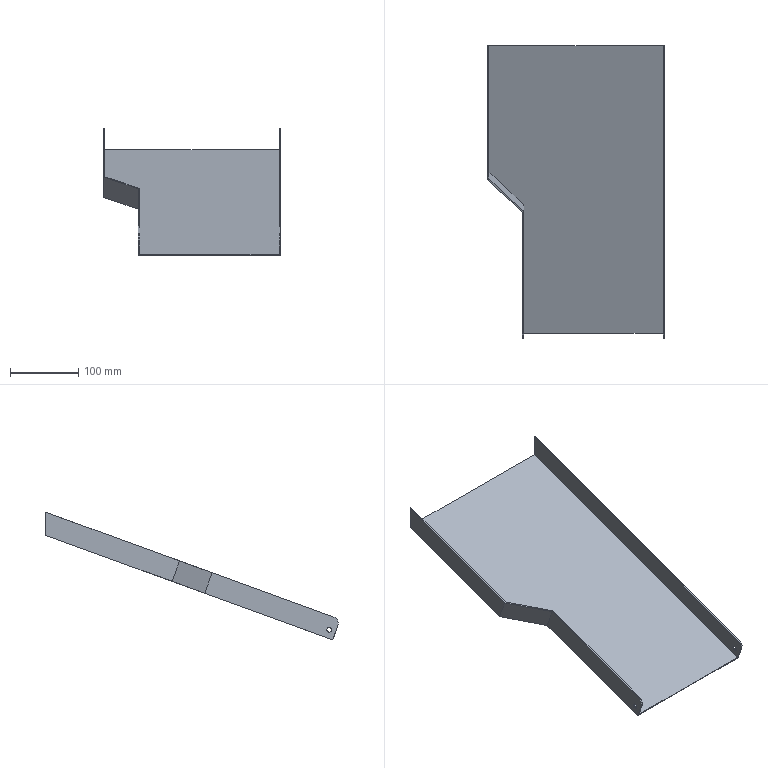Part | NX | features HB 2 | 1 solid | 18 faces | box 260 x 430.033 x 187.615 mm | volume 266275 mm3 | plane 14 | cylinder 4 | commonest cylinder face diameters 7 x2 20 x2
STEP:
#1=CARTESIAN_POINT('',(3672.,-269.,-204.418));
#2=VERTEX_POINT('',#1);
#3=CARTESIAN_POINT('',(3672.,-269.,-236.344));
#4=VERTEX_POINT('',#3);
#5=CARTESIAN_POINT('',(3672.,-269.,-276.603));
#6=DIRECTION('',(0.,0.,-1.));
#7=VECTOR('',#6,1000.);
#8=LINE('',#5,#7);
#9=EDGE_CURVE('',#2,#4,#8,.T.);
#10=ORIENTED_EDGE('',*,*,#9,.T.);
#11=CARTESIAN_POINT('',(3928.,-269.,-236.344));
#12=VERTEX_POINT('',#11);
#13=CARTESIAN_POINT('',(3698.,-269.,-236.344));
#14=DIRECTION('',(1.,0.,0.));
#15=VECTOR('',#14,1000.);
#16=LINE('',#13,#15);
#17=EDGE_CURVE('',#4,#12,#16,.T.);
#18=ORIENTED_EDGE('',*,*,#17,.T.);
#19=CARTESIAN_POINT('',(3928.,-269.,-204.418));
#20=VERTEX_POINT('',#19);
#21=CARTESIAN_POINT('',(3928.,-269.,-276.603));
#22=DIRECTION('',(0.,0.,1.));
#23=VECTOR('',#22,1000.);
#24=LINE('',#21,#23);
#25=EDGE_CURVE('',#12,#20,#24,.T.);
#26=ORIENTED_EDGE('',*,*,#25,.T.);
#27=CARTESIAN_POINT('',(3930.,-269.,-204.418));
#28=VERTEX_POINT('',#27);
#29=CARTESIAN_POINT('',(3930.,-269.,-204.418));
#30=DIRECTION('',(-1.,0.,0.));
#31=VECTOR('',#30,1000.);
#32=LINE('',#29,#31);
#33=EDGE_CURVE('',#28,#20,#32,.T.);
#34=ORIENTED_EDGE('',*,*,#33,.F.);
#35=CARTESIAN_POINT('',(3930.,-269.,-238.472));
#36=VERTEX_POINT('',#35);
#37=CARTESIAN_POINT('',(3930.,-269.,-276.603));
#38=DIRECTION('',(0.,0.,1.));
#39=VECTOR('',#38,1000.);
#40=LINE('',#37,#39);
#41=EDGE_CURVE('',#36,#28,#40,.T.);
#42=ORIENTED_EDGE('',*,*,#41,.F.);
#43=CARTESIAN_POINT('',(3670.,-269.,-238.472));
#44=VERTEX_POINT('',#43);
#45=CARTESIAN_POINT('',(3698.,-269.,-238.472));
#46=DIRECTION('',(1.,0.,0.));
#47=VECTOR('',#46,1000.);
#48=LINE('',#45,#47);
#49=EDGE_CURVE('',#44,#36,#48,.T.);
#50=ORIENTED_EDGE('',*,*,#49,.F.);
#51=CARTESIAN_POINT('',(3670.,-269.,-204.418));
#52=VERTEX_POINT('',#51);
#53=CARTESIAN_POINT('',(3670.,-269.,-276.603));
#54=DIRECTION('',(0.,0.,-1.));
#55=VECTOR('',#54,1000.);
#56=LINE('',#53,#55);
#57=EDGE_CURVE('',#52,#44,#56,.T.);
#58=ORIENTED_EDGE('',*,*,#57,.F.);
#59=CARTESIAN_POINT('',(3603.,-269.,-204.418));
#60=DIRECTION('',(-1.,0.,0.));
#61=VECTOR('',#60,1000.);
#62=LINE('',#59,#61);
#63=EDGE_CURVE('',#2,#52,#62,.T.);
#64=ORIENTED_EDGE('',*,*,#63,.F.);
#65=EDGE_LOOP('',(#10,#18,#26,#34,#42,#50,#58,#64));
#66=FACE_BOUND('',#65,.T.);
#67=CARTESIAN_POINT('',(4322.,-269.,100.));
#68=DIRECTION('',(0.,1.,0.));
#69=DIRECTION('',(0.,0.,1.));
#70=AXIS2_PLACEMENT_3D('',#67,#68,#69);
#71=PLANE('',#70);
#72=ADVANCED_FACE('',(#66),#71,.T.);
#73=CARTESIAN_POINT('',(3723.,-502.577,-321.359));
#74=VERTEX_POINT('',#73);
#75=CARTESIAN_POINT('',(3672.,-454.652,-303.916));
#76=VERTEX_POINT('',#75);
#77=CARTESIAN_POINT('',(3645.071,-429.348,-294.705));
#78=DIRECTION('',(-0.7071,0.6645,0.2418));
#79=VECTOR('',#78,1000.);
#80=LINE('',#77,#79);
#81=EDGE_CURVE('',#74,#76,#80,.T.);
#82=ORIENTED_EDGE('',*,*,#81,.F.);
#83=CARTESIAN_POINT('',(3723.,-691.589,-390.154));
#84=VERTEX_POINT('',#83);
#85=CARTESIAN_POINT('',(3723.,-379.611,-276.603));
#86=DIRECTION('',(0.,0.9397,0.342));
#87=VECTOR('',#86,1000.);
#88=LINE('',#85,#87);
#89=EDGE_CURVE('',#84,#74,#88,.T.);
#90=ORIENTED_EDGE('',*,*,#89,.F.);
#91=CARTESIAN_POINT('',(3928.,-691.589,-390.154));
#92=VERTEX_POINT('',#91);
#93=CARTESIAN_POINT('',(3698.,-691.589,-390.154));
#94=DIRECTION('',(1.,0.,0.));
#95=VECTOR('',#94,1000.);
#96=LINE('',#93,#95);
#97=EDGE_CURVE('',#84,#92,#96,.T.);
#98=ORIENTED_EDGE('',*,*,#97,.T.);
#99=CARTESIAN_POINT('',(3928.,-379.611,-276.603));
#100=DIRECTION('',(0.,-0.9397,-0.342));
#101=VECTOR('',#100,1000.);
#102=LINE('',#99,#101);
#103=EDGE_CURVE('',#12,#92,#102,.T.);
#104=ORIENTED_EDGE('',*,*,#103,.F.);
#105=ORIENTED_EDGE('',*,*,#17,.F.);
#106=CARTESIAN_POINT('',(3672.,-379.611,-276.603));
#107=DIRECTION('',(0.,0.9397,0.342));
#108=VECTOR('',#107,1000.);
#109=LINE('',#106,#108);
#110=EDGE_CURVE('',#76,#4,#109,.T.);
#111=ORIENTED_EDGE('',*,*,#110,.F.);
#112=EDGE_LOOP('',(#82,#90,#98,#104,#105,#111));
#113=FACE_BOUND('',#112,.T.);
#114=CARTESIAN_POINT('',(3698.,-379.611,-276.603));
#115=DIRECTION('',(0.,-0.342,0.9397));
#116=DIRECTION('',(1.,0.,0.));
#117=AXIS2_PLACEMENT_3D('',#114,#115,#116);
#118=PLANE('',#117);
#119=ADVANCED_FACE('',(#113),#118,.T.);
#120=CARTESIAN_POINT('',(3672.,-464.913,-275.725));
#121=VERTEX_POINT('',#120);
#122=CARTESIAN_POINT('',(3672.,-464.913,-275.725));
#123=DIRECTION('',(0.,0.342,-0.9397));
#124=VECTOR('',#123,1000.);
#125=LINE('',#122,#124);
#126=EDGE_CURVE('',#121,#76,#125,.T.);
#127=ORIENTED_EDGE('',*,*,#126,.T.);
#128=ORIENTED_EDGE('',*,*,#110,.T.);
#129=ORIENTED_EDGE('',*,*,#9,.F.);
#130=CARTESIAN_POINT('',(3672.,-389.872,-248.412));
#131=DIRECTION('',(0.,0.9397,0.342));
#132=VECTOR('',#131,1000.);
#133=LINE('',#130,#132);
#134=EDGE_CURVE('',#121,#2,#133,.T.);
#135=ORIENTED_EDGE('',*,*,#134,.F.);
#136=EDGE_LOOP('',(#127,#128,#129,#135));
#137=FACE_BOUND('',#136,.T.);
#138=CARTESIAN_POINT('',(3672.,-379.611,-276.603));
#139=DIRECTION('',(1.,0.,0.));
#140=DIRECTION('',(0.,0.08716,0.9962));
#141=AXIS2_PLACEMENT_3D('',#138,#139,#140);
#142=PLANE('',#141);
#143=ADVANCED_FACE('',(#137),#142,.T.);
#144=CARTESIAN_POINT('',(3930.,-692.453,-358.543));
#145=VERTEX_POINT('',#144);
#146=CARTESIAN_POINT('',(3930.,-389.872,-248.412));
#147=DIRECTION('',(0.,0.9397,0.342));
#148=VECTOR('',#147,1000.);
#149=LINE('',#146,#148);
#150=EDGE_CURVE('',#145,#28,#149,.T.);
#151=ORIENTED_EDGE('',*,*,#150,.F.);
#152=CARTESIAN_POINT('',(3930.,-698.43,-371.36));
#153=VERTEX_POINT('',#152);
#154=CARTESIAN_POINT('',(3930.,-689.033,-367.939));
#155=DIRECTION('',(1.,0.,0.));
#156=DIRECTION('',(0.,0.,1.));
#157=AXIS2_PLACEMENT_3D('',#154,#155,#156);
#158=CIRCLE('',#157,10.);
#159=EDGE_CURVE('',#145,#153,#158,.T.);
#160=ORIENTED_EDGE('',*,*,#159,.T.);
#161=CARTESIAN_POINT('',(3930.,-690.905,-392.033));
#162=VERTEX_POINT('',#161);
#163=CARTESIAN_POINT('',(3930.,-691.589,-390.154));
#164=DIRECTION('',(0.,-0.342,0.9397));
#165=VECTOR('',#164,1000.);
#166=LINE('',#163,#165);
#167=EDGE_CURVE('',#162,#153,#166,.T.);
#168=ORIENTED_EDGE('',*,*,#167,.F.);
#169=CARTESIAN_POINT('',(3930.,-378.927,-278.482));
#170=DIRECTION('',(0.,0.9397,0.342));
#171=VECTOR('',#170,1000.);
#172=LINE('',#169,#171);
#173=EDGE_CURVE('',#162,#36,#172,.T.);
#174=ORIENTED_EDGE('',*,*,#173,.T.);
#175=ORIENTED_EDGE('',*,*,#41,.T.);
#176=EDGE_LOOP('',(#151,#160,#168,#174,#175));
#177=FACE_BOUND('',#176,.T.);
#178=CARTESIAN_POINT('',(3930.,-685.612,-373.836));
#179=VERTEX_POINT('',#178);
#180=CARTESIAN_POINT('',(3930.,-685.612,-377.336));
#181=DIRECTION('',(-1.,0.,0.));
#182=DIRECTION('',(0.,0.,1.));
#183=AXIS2_PLACEMENT_3D('',#180,#181,#182);
#184=CIRCLE('',#183,3.5);
#185=EDGE_CURVE('',#179,#179,#184,.T.);
#186=ORIENTED_EDGE('',*,*,#185,.T.);
#187=EDGE_LOOP('',(#186));
#188=FACE_BOUND('',#187,.T.);
#189=CARTESIAN_POINT('',(3930.,-379.611,-276.603));
#190=DIRECTION('',(-1.,0.,0.));
#191=DIRECTION('',(0.,0.08716,0.9962));
#192=AXIS2_PLACEMENT_3D('',#189,#190,#191);
#193=PLANE('',#192);
#194=ADVANCED_FACE('',(#177,#188),#193,.F.);
#195=CARTESIAN_POINT('',(3928.,-692.453,-358.543));
#196=VERTEX_POINT('',#195);
#197=CARTESIAN_POINT('',(3928.,-389.872,-248.412));
#198=DIRECTION('',(0.,0.9397,0.342));
#199=VECTOR('',#198,1000.);
#200=LINE('',#197,#199);
#201=EDGE_CURVE('',#196,#20,#200,.T.);
#202=ORIENTED_EDGE('',*,*,#201,.F.);
#203=CARTESIAN_POINT('',(3875.,-692.453,-358.543));
#204=DIRECTION('',(1.,0.,0.));
#205=VECTOR('',#204,1000.);
#206=LINE('',#203,#205);
#207=EDGE_CURVE('',#196,#145,#206,.T.);
#208=ORIENTED_EDGE('',*,*,#207,.T.);
#209=ORIENTED_EDGE('',*,*,#150,.T.);
#210=ORIENTED_EDGE('',*,*,#33,.T.);
#211=EDGE_LOOP('',(#202,#208,#209,#210));
#212=FACE_BOUND('',#211,.T.);
#213=CARTESIAN_POINT('',(3930.,-389.872,-248.412));
#214=DIRECTION('',(0.,0.342,-0.9397));
#215=DIRECTION('',(0.,-0.9397,-0.342));
#216=AXIS2_PLACEMENT_3D('',#213,#214,#215);
#217=PLANE('',#216);
#218=ADVANCED_FACE('',(#212),#217,.F.);
#219=CARTESIAN_POINT('',(3721.,-502.671,-323.521));
#220=VERTEX_POINT('',#219);
#221=CARTESIAN_POINT('',(3721.,-690.905,-392.033));
#222=VERTEX_POINT('',#221);
#223=CARTESIAN_POINT('',(3721.,-378.927,-278.482));
#224=DIRECTION('',(0.,-0.9397,-0.342));
#225=VECTOR('',#224,1000.);
#226=LINE('',#223,#225);
#227=EDGE_CURVE('',#220,#222,#226,.T.);
#228=ORIENTED_EDGE('',*,*,#227,.F.);
#229=CARTESIAN_POINT('',(3670.,-454.747,-306.078));
#230=VERTEX_POINT('',#229);
#231=CARTESIAN_POINT('',(3643.657,-429.993,-297.069));
#232=DIRECTION('',(-0.7071,0.6645,0.2418));
#233=VECTOR('',#232,1000.);
#234=LINE('',#231,#233);
#235=EDGE_CURVE('',#220,#230,#234,.T.);
#236=ORIENTED_EDGE('',*,*,#235,.T.);
#237=CARTESIAN_POINT('',(3670.,-378.927,-278.482));
#238=DIRECTION('',(0.,-0.9397,-0.342));
#239=VECTOR('',#238,1000.);
#240=LINE('',#237,#239);
#241=EDGE_CURVE('',#44,#230,#240,.T.);
#242=ORIENTED_EDGE('',*,*,#241,.F.);
#243=ORIENTED_EDGE('',*,*,#49,.T.);
#244=ORIENTED_EDGE('',*,*,#173,.F.);
#245=CARTESIAN_POINT('',(3698.,-690.905,-392.033));
#246=DIRECTION('',(1.,0.,0.));
#247=VECTOR('',#246,1000.);
#248=LINE('',#245,#247);
#249=EDGE_CURVE('',#222,#162,#248,.T.);
#250=ORIENTED_EDGE('',*,*,#249,.F.);
#251=EDGE_LOOP('',(#228,#236,#242,#243,#244,#250));
#252=FACE_BOUND('',#251,.T.);
#253=CARTESIAN_POINT('',(3698.,-378.927,-278.482));
#254=DIRECTION('',(0.,-0.342,0.9397));
#255=DIRECTION('',(1.,0.,0.));
#256=AXIS2_PLACEMENT_3D('',#253,#254,#255);
#257=PLANE('',#256);
#258=ADVANCED_FACE('',(#252),#257,.F.);
#259=ORIENTED_EDGE('',*,*,#241,.T.);
#260=CARTESIAN_POINT('',(3670.,-465.691,-276.008));
#261=VERTEX_POINT('',#260);
#262=CARTESIAN_POINT('',(3670.,-465.691,-276.008));
#263=DIRECTION('',(0.,0.342,-0.9397));
#264=VECTOR('',#263,1000.);
#265=LINE('',#262,#264);
#266=EDGE_CURVE('',#261,#230,#265,.T.);
#267=ORIENTED_EDGE('',*,*,#266,.F.);
#268=CARTESIAN_POINT('',(3670.,-389.872,-248.412));
#269=DIRECTION('',(0.,0.9397,0.342));
#270=VECTOR('',#269,1000.);
#271=LINE('',#268,#270);
#272=EDGE_CURVE('',#261,#52,#271,.T.);
#273=ORIENTED_EDGE('',*,*,#272,.T.);
#274=ORIENTED_EDGE('',*,*,#57,.T.);
#275=EDGE_LOOP('',(#259,#267,#273,#274));
#276=FACE_BOUND('',#275,.T.);
#277=CARTESIAN_POINT('',(3670.,-379.611,-276.603));
#278=DIRECTION('',(1.,0.,0.));
#279=DIRECTION('',(0.,-0.08716,-0.9962));
#280=AXIS2_PLACEMENT_3D('',#277,#278,#279);
#281=PLANE('',#280);
#282=ADVANCED_FACE('',(#276),#281,.F.);
#283=CARTESIAN_POINT('',(3721.,-513.616,-293.451));
#284=VERTEX_POINT('',#283);
#285=CARTESIAN_POINT('',(3596.157,-396.302,-250.752));
#286=DIRECTION('',(0.7071,-0.6645,-0.2418));
#287=VECTOR('',#286,1000.);
#288=LINE('',#285,#287);
#289=EDGE_CURVE('',#261,#284,#288,.T.);
#290=ORIENTED_EDGE('',*,*,#289,.T.);
#291=CARTESIAN_POINT('',(3721.,-692.453,-358.543));
#292=VERTEX_POINT('',#291);
#293=CARTESIAN_POINT('',(3721.,-389.872,-248.412));
#294=DIRECTION('',(0.,0.9397,0.342));
#295=VECTOR('',#294,1000.);
#296=LINE('',#293,#295);
#297=EDGE_CURVE('',#292,#284,#296,.T.);
#298=ORIENTED_EDGE('',*,*,#297,.F.);
#299=CARTESIAN_POINT('',(3723.,-692.453,-358.543));
#300=VERTEX_POINT('',#299);
#301=CARTESIAN_POINT('',(3603.,-692.453,-358.543));
#302=DIRECTION('',(1.,0.,0.));
#303=VECTOR('',#302,1000.);
#304=LINE('',#301,#303);
#305=EDGE_CURVE('',#292,#300,#304,.T.);
#306=ORIENTED_EDGE('',*,*,#305,.T.);
#307=CARTESIAN_POINT('',(3723.,-512.837,-293.168));
#308=VERTEX_POINT('',#307);
#309=CARTESIAN_POINT('',(3723.,-389.872,-248.412));
#310=DIRECTION('',(0.,0.9397,0.342));
#311=VECTOR('',#310,1000.);
#312=LINE('',#309,#311);
#313=EDGE_CURVE('',#300,#308,#312,.T.);
#314=ORIENTED_EDGE('',*,*,#313,.T.);
#315=CARTESIAN_POINT('',(3597.571,-394.973,-250.269));
#316=DIRECTION('',(0.7071,-0.6645,-0.2418));
#317=VECTOR('',#316,1000.);
#318=LINE('',#315,#317);
#319=EDGE_CURVE('',#121,#308,#318,.T.);
#320=ORIENTED_EDGE('',*,*,#319,.F.);
#321=ORIENTED_EDGE('',*,*,#134,.T.);
#322=ORIENTED_EDGE('',*,*,#63,.T.);
#323=ORIENTED_EDGE('',*,*,#272,.F.);
#324=EDGE_LOOP('',(#290,#298,#306,#314,#320,#321,#322,#323));
#325=FACE_BOUND('',#324,.T.);
#326=CARTESIAN_POINT('',(3603.,-389.872,-248.412));
#327=DIRECTION('',(0.,0.342,-0.9397));
#328=DIRECTION('',(0.,-0.9397,-0.342));
#329=AXIS2_PLACEMENT_3D('',#326,#327,#328);
#330=PLANE('',#329);
#331=ADVANCED_FACE('',(#325),#330,.F.);
#332=ORIENTED_EDGE('',*,*,#103,.T.);
#333=CARTESIAN_POINT('',(3928.,-698.43,-371.36));
#334=VERTEX_POINT('',#333);
#335=CARTESIAN_POINT('',(3928.,-691.589,-390.154));
#336=DIRECTION('',(0.,-0.342,0.9397));
#337=VECTOR('',#336,1000.);
#338=LINE('',#335,#337);
#339=EDGE_CURVE('',#92,#334,#338,.T.);
#340=ORIENTED_EDGE('',*,*,#339,.T.);
#341=CARTESIAN_POINT('',(3928.,-689.033,-367.939));
#342=DIRECTION('',(-1.,0.,0.));
#343=DIRECTION('',(0.,0.,1.));
#344=AXIS2_PLACEMENT_3D('',#341,#342,#343);
#345=CIRCLE('',#344,10.);
#346=EDGE_CURVE('',#334,#196,#345,.T.);
#347=ORIENTED_EDGE('',*,*,#346,.T.);
#348=ORIENTED_EDGE('',*,*,#201,.T.);
#349=ORIENTED_EDGE('',*,*,#25,.F.);
#350=EDGE_LOOP('',(#332,#340,#347,#348,#349));
#351=FACE_BOUND('',#350,.T.);
#352=CARTESIAN_POINT('',(3928.,-685.612,-373.836));
#353=VERTEX_POINT('',#352);
#354=CARTESIAN_POINT('',(3928.,-685.612,-377.336));
#355=DIRECTION('',(1.,0.,0.));
#356=DIRECTION('',(0.,0.,1.));
#357=AXIS2_PLACEMENT_3D('',#354,#355,#356);
#358=CIRCLE('',#357,3.5);
#359=EDGE_CURVE('',#353,#353,#358,.T.);
#360=ORIENTED_EDGE('',*,*,#359,.T.);
#361=EDGE_LOOP('',(#360));
#362=FACE_BOUND('',#361,.T.);
#363=CARTESIAN_POINT('',(3928.,-379.611,-276.603));
#364=DIRECTION('',(-1.,0.,0.));
#365=DIRECTION('',(0.,0.08716,0.9962));
#366=AXIS2_PLACEMENT_3D('',#363,#364,#365);
#367=PLANE('',#366);
#368=ADVANCED_FACE('',(#351,#362),#367,.T.);
#369=CARTESIAN_POINT('',(3723.,-685.307,-373.85));
#370=VERTEX_POINT('',#369);
#371=CARTESIAN_POINT('',(3723.,-685.612,-377.336));
#372=DIRECTION('',(-1.,0.,0.));
#373=DIRECTION('',(0.,0.08716,0.9962));
#374=AXIS2_PLACEMENT_3D('',#371,#372,#373);
#375=CIRCLE('',#374,3.5);
#376=EDGE_CURVE('',#370,#370,#375,.T.);
#377=ORIENTED_EDGE('',*,*,#376,.T.);
#378=EDGE_LOOP('',(#377));
#379=FACE_BOUND('',#378,.T.);
#380=ORIENTED_EDGE('',*,*,#89,.T.);
#381=CARTESIAN_POINT('',(3723.,-502.577,-321.359));
#382=DIRECTION('',(0.,-0.342,0.9397));
#383=VECTOR('',#382,1000.);
#384=LINE('',#381,#383);
#385=EDGE_CURVE('',#74,#308,#384,.T.);
#386=ORIENTED_EDGE('',*,*,#385,.T.);
#387=ORIENTED_EDGE('',*,*,#313,.F.);
#388=CARTESIAN_POINT('',(3723.,-698.43,-371.36));
#389=VERTEX_POINT('',#388);
#390=CARTESIAN_POINT('',(3723.,-689.033,-367.939));
#391=DIRECTION('',(1.,0.,0.));
#392=DIRECTION('',(0.,0.08716,0.9962));
#393=AXIS2_PLACEMENT_3D('',#390,#391,#392);
#394=CIRCLE('',#393,10.);
#395=EDGE_CURVE('',#300,#389,#394,.T.);
#396=ORIENTED_EDGE('',*,*,#395,.T.);
#397=CARTESIAN_POINT('',(3723.,-691.589,-390.154));
#398=DIRECTION('',(0.,-0.342,0.9397));
#399=VECTOR('',#398,1000.);
#400=LINE('',#397,#399);
#401=EDGE_CURVE('',#84,#389,#400,.T.);
#402=ORIENTED_EDGE('',*,*,#401,.F.);
#403=EDGE_LOOP('',(#380,#386,#387,#396,#402));
#404=FACE_BOUND('',#403,.T.);
#405=CARTESIAN_POINT('',(3723.,-379.611,-276.603));
#406=DIRECTION('',(1.,0.,0.));
#407=DIRECTION('',(0.,0.08716,0.9962));
#408=AXIS2_PLACEMENT_3D('',#405,#406,#407);
#409=PLANE('',#408);
#410=ADVANCED_FACE('',(#379,#404),#409,.T.);
#411=CARTESIAN_POINT('',(3721.,-685.307,-373.85));
#412=VERTEX_POINT('',#411);
#413=CARTESIAN_POINT('',(3721.,-685.612,-377.336));
#414=DIRECTION('',(-1.,0.,0.));
#415=DIRECTION('',(0.,0.08716,0.9962));
#416=AXIS2_PLACEMENT_3D('',#413,#414,#415);
#417=CIRCLE('',#416,3.5);
#418=EDGE_CURVE('',#412,#412,#417,.T.);
#419=ORIENTED_EDGE('',*,*,#418,.F.);
#420=EDGE_LOOP('',(#419));
#421=FACE_BOUND('',#420,.T.);
#422=CARTESIAN_POINT('',(3721.,-503.355,-321.642));
#423=DIRECTION('',(0.,-0.342,0.9397));
#424=VECTOR('',#423,1000.);
#425=LINE('',#422,#424);
#426=EDGE_CURVE('',#220,#284,#425,.T.);
#427=ORIENTED_EDGE('',*,*,#426,.F.);
#428=ORIENTED_EDGE('',*,*,#227,.T.);
#429=CARTESIAN_POINT('',(3721.,-698.43,-371.36));
#430=VERTEX_POINT('',#429);
#431=CARTESIAN_POINT('',(3721.,-691.589,-390.154));
#432=DIRECTION('',(0.,-0.342,0.9397));
#433=VECTOR('',#432,1000.);
#434=LINE('',#431,#433);
#435=EDGE_CURVE('',#222,#430,#434,.T.);
#436=ORIENTED_EDGE('',*,*,#435,.T.);
#437=CARTESIAN_POINT('',(3721.,-689.033,-367.939));
#438=DIRECTION('',(-1.,0.,0.));
#439=DIRECTION('',(0.,0.08716,0.9962));
#440=AXIS2_PLACEMENT_3D('',#437,#438,#439);
#441=CIRCLE('',#440,10.);
#442=EDGE_CURVE('',#430,#292,#441,.T.);
#443=ORIENTED_EDGE('',*,*,#442,.T.);
#444=ORIENTED_EDGE('',*,*,#297,.T.);
#445=EDGE_LOOP('',(#427,#428,#436,#443,#444));
#446=FACE_BOUND('',#445,.T.);
#447=CARTESIAN_POINT('',(3721.,-379.611,-276.603));
#448=DIRECTION('',(1.,0.,0.));
#449=DIRECTION('',(0.,-0.08716,-0.9962));
#450=AXIS2_PLACEMENT_3D('',#447,#448,#449);
#451=PLANE('',#450);
#452=ADVANCED_FACE('',(#421,#446),#451,.F.);
#453=ORIENTED_EDGE('',*,*,#376,.F.);
#454=EDGE_LOOP('',(#453));
#455=FACE_BOUND('',#454,.T.);
#456=ORIENTED_EDGE('',*,*,#418,.T.);
#457=EDGE_LOOP('',(#456));
#458=FACE_BOUND('',#457,.T.);
#459=CARTESIAN_POINT('',(2999.,-685.612,-377.336));
#460=DIRECTION('',(1.,0.,0.));
#461=DIRECTION('',(0.,-0.08716,-0.9962));
#462=AXIS2_PLACEMENT_3D('',#459,#460,#461);
#463=CYLINDRICAL_SURFACE('',#462,3.5);
#464=ADVANCED_FACE('',(#455,#458),#463,.F.);
#465=ORIENTED_EDGE('',*,*,#395,.F.);
#466=ORIENTED_EDGE('',*,*,#305,.F.);
#467=ORIENTED_EDGE('',*,*,#442,.F.);
#468=CARTESIAN_POINT('',(3603.,-698.43,-371.36));
#469=DIRECTION('',(-1.,0.,0.));
#470=VECTOR('',#469,1000.);
#471=LINE('',#468,#470);
#472=EDGE_CURVE('',#389,#430,#471,.T.);
#473=ORIENTED_EDGE('',*,*,#472,.F.);
#474=EDGE_LOOP('',(#465,#466,#467,#473));
#475=FACE_BOUND('',#474,.T.);
#476=CARTESIAN_POINT('',(3603.,-689.033,-367.939));
#477=DIRECTION('',(-1.,0.,0.));
#478=DIRECTION('',(0.,0.08716,0.9962));
#479=AXIS2_PLACEMENT_3D('',#476,#477,#478);
#480=CYLINDRICAL_SURFACE('',#479,10.);
#481=ADVANCED_FACE('',(#475),#480,.T.);
#482=ORIENTED_EDGE('',*,*,#97,.F.);
#483=ORIENTED_EDGE('',*,*,#401,.T.);
#484=ORIENTED_EDGE('',*,*,#472,.T.);
#485=ORIENTED_EDGE('',*,*,#435,.F.);
#486=ORIENTED_EDGE('',*,*,#249,.T.);
#487=ORIENTED_EDGE('',*,*,#167,.T.);
#488=CARTESIAN_POINT('',(3617.,-698.43,-371.36));
#489=DIRECTION('',(-1.,0.,0.));
#490=VECTOR('',#489,1000.);
#491=LINE('',#488,#490);
#492=EDGE_CURVE('',#153,#334,#491,.T.);
#493=ORIENTED_EDGE('',*,*,#492,.T.);
#494=ORIENTED_EDGE('',*,*,#339,.F.);
#495=EDGE_LOOP('',(#482,#483,#484,#485,#486,#487,#493,#494));
#496=FACE_BOUND('',#495,.T.);
#497=CARTESIAN_POINT('',(3698.,-691.589,-390.154));
#498=DIRECTION('',(0.,0.9397,0.342));
#499=DIRECTION('',(0.,0.342,-0.9397));
#500=AXIS2_PLACEMENT_3D('',#497,#498,#499);
#501=PLANE('',#500);
#502=ADVANCED_FACE('',(#496),#501,.F.);
#503=ORIENTED_EDGE('',*,*,#346,.F.);
#504=ORIENTED_EDGE('',*,*,#492,.F.);
#505=ORIENTED_EDGE('',*,*,#159,.F.);
#506=ORIENTED_EDGE('',*,*,#207,.F.);
#507=EDGE_LOOP('',(#503,#504,#505,#506));
#508=FACE_BOUND('',#507,.T.);
#509=CARTESIAN_POINT('',(3617.,-689.033,-367.939));
#510=DIRECTION('',(1.,0.,0.));
#511=DIRECTION('',(0.,-0.08716,-0.9962));
#512=AXIS2_PLACEMENT_3D('',#509,#510,#511);
#513=CYLINDRICAL_SURFACE('',#512,10.);
#514=ADVANCED_FACE('',(#508),#513,.T.);
#515=ORIENTED_EDGE('',*,*,#359,.F.);
#516=EDGE_LOOP('',(#515));
#517=FACE_BOUND('',#516,.T.);
#518=ORIENTED_EDGE('',*,*,#185,.F.);
#519=EDGE_LOOP('',(#518));
#520=FACE_BOUND('',#519,.T.);
#521=CARTESIAN_POINT('',(3025.,-685.612,-377.336));
#522=DIRECTION('',(1.,0.,0.));
#523=DIRECTION('',(0.,-0.08716,-0.9962));
#524=AXIS2_PLACEMENT_3D('',#521,#522,#523);
#525=CYLINDRICAL_SURFACE('',#524,3.5);
#526=ADVANCED_FACE('',(#517,#520),#525,.F.);
#527=ORIENTED_EDGE('',*,*,#235,.F.);
#528=ORIENTED_EDGE('',*,*,#426,.T.);
#529=ORIENTED_EDGE('',*,*,#289,.F.);
#530=ORIENTED_EDGE('',*,*,#266,.T.);
#531=EDGE_LOOP('',(#527,#528,#529,#530));
#532=FACE_BOUND('',#531,.T.);
#533=CARTESIAN_POINT('',(3671.,-466.631,-276.35));
#534=DIRECTION('',(-0.7071,-0.6645,-0.2418));
#535=DIRECTION('',(0.,-0.342,0.9397));
#536=AXIS2_PLACEMENT_3D('',#533,#534,#535);
#537=PLANE('',#536);
#538=ADVANCED_FACE('',(#532),#537,.T.);
#539=ORIENTED_EDGE('',*,*,#385,.F.);
#540=ORIENTED_EDGE('',*,*,#81,.T.);
#541=ORIENTED_EDGE('',*,*,#126,.F.);
#542=ORIENTED_EDGE('',*,*,#319,.T.);
#543=EDGE_LOOP('',(#539,#540,#541,#542));
#544=FACE_BOUND('',#543,.T.);
#545=CARTESIAN_POINT('',(3672.414,-465.302,-275.866));
#546=DIRECTION('',(-0.7071,-0.6645,-0.2418));
#547=DIRECTION('',(0.,-0.342,0.9397));
#548=AXIS2_PLACEMENT_3D('',#545,#546,#547);
#549=PLANE('',#548);
#550=ADVANCED_FACE('',(#544),#549,.F.);
#551=CLOSED_SHELL('',(#72,#119,#143,#194,#218,#258,#282,#331,#368,#410,#452,#464,#481,#502,#514,#526,#538,#550));
#552=MANIFOLD_SOLID_BREP('',#551);
#553=(LENGTH_UNIT()NAMED_UNIT(*)SI_UNIT(.MILLI.,.METRE.));
#554=UNCERTAINTY_MEASURE_WITH_UNIT(LENGTH_MEASURE(0.00001),#553,'','');
#555=(NAMED_UNIT(*)PLANE_ANGLE_UNIT()SI_UNIT($,.RADIAN.));
#556=(NAMED_UNIT(*)SI_UNIT($,.STERADIAN.)SOLID_ANGLE_UNIT());
#557=(GEOMETRIC_REPRESENTATION_CONTEXT(3)GLOBAL_UNCERTAINTY_ASSIGNED_CONTEXT((#554))GLOBAL_UNIT_ASSIGNED_CONTEXT((#553,#555,#556))REPRESENTATION_CONTEXT('',''));
#558=ADVANCED_BREP_SHAPE_REPRESENTATION('',(#552),#557);